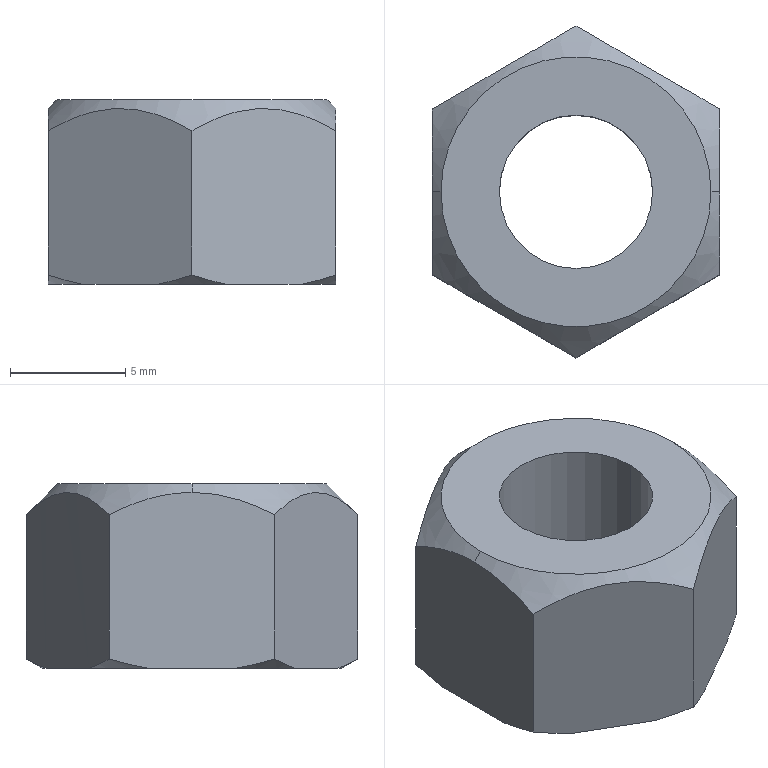Part | SolidWorks | features MBimport 1 | 1 solid | 20 faces | box 12.454 x 14.38 x 8 mm | volume 784.997 mm3 | cone 10 | plane 8 | cylinder 2 | commonest cylinder face diameters 6.647 x2
STEP:
#1=CARTESIAN_POINT('',(-5.85,0.,8.));
#2=VERTEX_POINT('',#1);
#3=CARTESIAN_POINT('',(-6.227,0.,7.623));
#4=VERTEX_POINT('',#3);
#5=CARTESIAN_POINT('',(-5.85,0.,8.));
#6=DIRECTION('',(-0.7071,0.,-0.7071));
#7=VECTOR('',#6,1000.);
#8=LINE('',#5,#7);
#9=EDGE_CURVE('',#2,#4,#8,.T.);
#10=ORIENTED_EDGE('',*,*,#9,.F.);
#11=CARTESIAN_POINT('',(5.85,0.,8.));
#12=VERTEX_POINT('',#11);
#13=CARTESIAN_POINT('',(0.,0.,8.));
#14=DIRECTION('',(0.,0.,1.));
#15=DIRECTION('',(1.,0.,0.));
#16=AXIS2_PLACEMENT_3D('',#13,#14,#15);
#17=CIRCLE('',#16,5.85);
#18=EDGE_CURVE('',#12,#2,#17,.T.);
#19=ORIENTED_EDGE('',*,*,#18,.F.);
#20=CARTESIAN_POINT('',(6.227,0.,7.623));
#21=VERTEX_POINT('',#20);
#22=CARTESIAN_POINT('',(5.85,0.,8.));
#23=DIRECTION('',(0.7071,0.,-0.7071));
#24=VECTOR('',#23,1000.);
#25=LINE('',#22,#24);
#26=EDGE_CURVE('',#12,#21,#25,.T.);
#27=ORIENTED_EDGE('',*,*,#26,.T.);
#28=CARTESIAN_POINT('',(6.227,3.595,6.66));
#29=VERTEX_POINT('',#28);
#30=CARTESIAN_POINT('',(6.227,0.,7.623));
#31=CARTESIAN_POINT('',(6.227,0.1561,7.623));
#32=CARTESIAN_POINT('',(6.227,0.3116,7.617));
#33=CARTESIAN_POINT('',(6.227,0.5452,7.6));
#34=CARTESIAN_POINT('',(6.227,0.6621,7.589));
#35=CARTESIAN_POINT('',(6.227,0.7794,7.575));
#36=CARTESIAN_POINT('',(6.227,0.8577,7.565));
#37=CARTESIAN_POINT('',(6.227,0.8982,7.559));
#38=CARTESIAN_POINT('',(6.227,1.088,7.531));
#39=CARTESIAN_POINT('',(6.227,1.24,7.503));
#40=CARTESIAN_POINT('',(6.227,1.468,7.453));
#41=CARTESIAN_POINT('',(6.227,1.582,7.426));
#42=CARTESIAN_POINT('',(6.227,1.716,7.391));
#43=CARTESIAN_POINT('',(6.227,1.774,7.376));
#44=CARTESIAN_POINT('',(6.227,1.812,7.365));
#45=CARTESIAN_POINT('',(6.227,1.833,7.359));
#46=CARTESIAN_POINT('',(6.227,2.421,7.192));
#47=CARTESIAN_POINT('',(6.227,2.994,6.96));
#48=CARTESIAN_POINT('',(6.227,3.595,6.66));
#49=B_SPLINE_CURVE_WITH_KNOTS('',3,(#30,#31,#32,#33,#34,#35,#36,#37,#38,#39,#40,#41,#42,#43,#44,#45,#46,#47,#48),.UNSPECIFIED.,.F.,.F.,(4,2,1,2,2,2,1,1,2,2,4),(0.,0.125,0.1875,0.2187,0.25,0.375,0.4375,0.4687,0.4844,0.5,1.),.UNSPECIFIED.);
#50=EDGE_CURVE('',#21,#29,#49,.T.);
#51=ORIENTED_EDGE('',*,*,#50,.T.);
#52=CARTESIAN_POINT('',(0.,7.19,6.66));
#53=VERTEX_POINT('',#52);
#54=CARTESIAN_POINT('',(6.227,3.595,6.66));
#55=CARTESIAN_POINT('',(5.969,3.744,6.809));
#56=CARTESIAN_POINT('',(5.716,3.89,6.941));
#57=CARTESIAN_POINT('',(5.343,4.105,7.114));
#58=CARTESIAN_POINT('',(5.219,4.177,7.167));
#59=CARTESIAN_POINT('',(5.034,4.283,7.24));
#60=CARTESIAN_POINT('',(4.942,4.337,7.276));
#61=CARTESIAN_POINT('',(4.835,4.399,7.314));
#62=CARTESIAN_POINT('',(4.789,4.425,7.33));
#63=CARTESIAN_POINT('',(4.758,4.443,7.34));
#64=CARTESIAN_POINT('',(4.744,4.451,7.345));
#65=CARTESIAN_POINT('',(4.595,4.537,7.394));
#66=CARTESIAN_POINT('',(4.464,4.613,7.433));
#67=CARTESIAN_POINT('',(4.267,4.726,7.483));
#68=CARTESIAN_POINT('',(4.169,4.783,7.506));
#69=CARTESIAN_POINT('',(4.071,4.84,7.526));
#70=CARTESIAN_POINT('',(4.005,4.877,7.539));
#71=CARTESIAN_POINT('',(3.974,4.896,7.545));
#72=CARTESIAN_POINT('',(3.803,4.994,7.574));
#73=CARTESIAN_POINT('',(3.668,5.072,7.592));
#74=CARTESIAN_POINT('',(3.396,5.229,7.617));
#75=CARTESIAN_POINT('',(3.26,5.308,7.623));
#76=CARTESIAN_POINT('',(2.99,5.464,7.624));
#77=CARTESIAN_POINT('',(2.856,5.541,7.618));
#78=CARTESIAN_POINT('',(2.654,5.658,7.601));
#79=CARTESIAN_POINT('',(2.587,5.697,7.594));
#80=CARTESIAN_POINT('',(2.452,5.775,7.577));
#81=CARTESIAN_POINT('',(2.382,5.815,7.567));
#82=CARTESIAN_POINT('',(2.184,5.929,7.533));
#83=CARTESIAN_POINT('',(2.052,6.006,7.505));
#84=CARTESIAN_POINT('',(1.853,6.12,7.456));
#85=CARTESIAN_POINT('',(1.753,6.178,7.429));
#86=CARTESIAN_POINT('',(1.637,6.245,7.394));
#87=CARTESIAN_POINT('',(1.587,6.274,7.379));
#88=CARTESIAN_POINT('',(1.554,6.293,7.368));
#89=CARTESIAN_POINT('',(1.536,6.303,7.362));
#90=CARTESIAN_POINT('',(1.023,6.599,7.195));
#91=CARTESIAN_POINT('',(0.5235,6.888,6.962));
#92=CARTESIAN_POINT('',(0.,7.19,6.66));
#93=B_SPLINE_CURVE_WITH_KNOTS('',3,(#54,#55,#56,#57,#58,#59,#60,#61,#62,#63,#64,#65,#66,#67,#68,#69,#70,#71,#72,#73,#74,#75,#76,#77,#78,#79,#80,#81,#82,#83,#84,#85,#86,#87,#88,#89,#90,#91,#92),.UNSPECIFIED.,.F.,.F.,(4,2,2,1,1,2,2,2,1,2,2,2,2,2,2,2,2,1,1,2,2,4),(0.,0.125,0.1875,0.2188,0.2344,0.2422,0.25,0.3125,0.3438,0.3594,0.375,0.4375,0.5,0.5625,0.5938,0.625,0.6875,0.7188,0.7344,0.7422,0.75,1.),.UNSPECIFIED.);
#94=EDGE_CURVE('',#29,#53,#93,.T.);
#95=ORIENTED_EDGE('',*,*,#94,.T.);
#96=CARTESIAN_POINT('',(-6.227,3.595,6.66));
#97=VERTEX_POINT('',#96);
#98=CARTESIAN_POINT('',(0.,7.19,6.66));
#99=CARTESIAN_POINT('',(-0.258,7.041,6.809));
#100=CARTESIAN_POINT('',(-0.5104,6.895,6.941));
#101=CARTESIAN_POINT('',(-0.884,6.679,7.114));
#102=CARTESIAN_POINT('',(-1.008,6.608,7.167));
#103=CARTESIAN_POINT('',(-1.192,6.501,7.24));
#104=CARTESIAN_POINT('',(-1.285,6.448,7.276));
#105=CARTESIAN_POINT('',(-1.392,6.386,7.314));
#106=CARTESIAN_POINT('',(-1.438,6.36,7.33));
#107=CARTESIAN_POINT('',(-1.469,6.342,7.34));
#108=CARTESIAN_POINT('',(-1.483,6.334,7.345));
#109=CARTESIAN_POINT('',(-1.632,6.248,7.394));
#110=CARTESIAN_POINT('',(-1.763,6.172,7.433));
#111=CARTESIAN_POINT('',(-1.96,6.059,7.483));
#112=CARTESIAN_POINT('',(-2.058,6.002,7.506));
#113=CARTESIAN_POINT('',(-2.156,5.945,7.526));
#114=CARTESIAN_POINT('',(-2.221,5.908,7.539));
#115=CARTESIAN_POINT('',(-2.253,5.889,7.545));
#116=CARTESIAN_POINT('',(-2.423,5.791,7.574));
#117=CARTESIAN_POINT('',(-2.559,5.712,7.592));
#118=CARTESIAN_POINT('',(-2.83,5.556,7.617));
#119=CARTESIAN_POINT('',(-2.967,5.477,7.623));
#120=CARTESIAN_POINT('',(-3.237,5.321,7.624));
#121=CARTESIAN_POINT('',(-3.371,5.244,7.618));
#122=CARTESIAN_POINT('',(-3.573,5.127,7.601));
#123=CARTESIAN_POINT('',(-3.64,5.088,7.594));
#124=CARTESIAN_POINT('',(-3.775,5.011,7.577));
#125=CARTESIAN_POINT('',(-3.844,4.971,7.567));
#126=CARTESIAN_POINT('',(-4.043,4.856,7.533));
#127=CARTESIAN_POINT('',(-4.175,4.78,7.505));
#128=CARTESIAN_POINT('',(-4.374,4.665,7.456));
#129=CARTESIAN_POINT('',(-4.473,4.607,7.429));
#130=CARTESIAN_POINT('',(-4.59,4.54,7.394));
#131=CARTESIAN_POINT('',(-4.64,4.511,7.379));
#132=CARTESIAN_POINT('',(-4.673,4.492,7.368));
#133=CARTESIAN_POINT('',(-4.691,4.482,7.362));
#134=CARTESIAN_POINT('',(-5.203,4.186,7.195));
#135=CARTESIAN_POINT('',(-5.703,3.897,6.962));
#136=CARTESIAN_POINT('',(-6.227,3.595,6.66));
#137=B_SPLINE_CURVE_WITH_KNOTS('',3,(#98,#99,#100,#101,#102,#103,#104,#105,#106,#107,#108,#109,#110,#111,#112,#113,#114,#115,#116,#117,#118,#119,#120,#121,#122,#123,#124,#125,#126,#127,#128,#129,#130,#131,#132,#133,#134,#135,#136),.UNSPECIFIED.,.F.,.F.,(4,2,2,1,1,2,2,2,1,2,2,2,2,2,2,2,2,1,1,2,2,4),(0.,0.125,0.1875,0.2187,0.2344,0.2422,0.25,0.3125,0.3437,0.3594,0.375,0.4375,0.5,0.5625,0.5937,0.625,0.6875,0.7187,0.7344,0.7422,0.75,1.),.UNSPECIFIED.);
#138=EDGE_CURVE('',#53,#97,#137,.T.);
#139=ORIENTED_EDGE('',*,*,#138,.T.);
#140=CARTESIAN_POINT('',(-6.227,3.595,6.66));
#141=CARTESIAN_POINT('',(-6.227,3.295,6.81));
#142=CARTESIAN_POINT('',(-6.227,3.001,6.943));
#143=CARTESIAN_POINT('',(-6.227,2.566,7.117));
#144=CARTESIAN_POINT('',(-6.227,2.422,7.17));
#145=CARTESIAN_POINT('',(-6.227,2.207,7.244));
#146=CARTESIAN_POINT('',(-6.227,2.1,7.279));
#147=CARTESIAN_POINT('',(-6.227,1.975,7.318));
#148=CARTESIAN_POINT('',(-6.227,1.922,7.334));
#149=CARTESIAN_POINT('',(-6.227,1.886,7.344));
#150=CARTESIAN_POINT('',(-6.227,1.87,7.349));
#151=CARTESIAN_POINT('',(-6.227,1.697,7.398));
#152=CARTESIAN_POINT('',(-6.227,1.544,7.436));
#153=CARTESIAN_POINT('',(-6.227,1.316,7.486));
#154=CARTESIAN_POINT('',(-6.227,1.202,7.509));
#155=CARTESIAN_POINT('',(-6.227,1.088,7.529));
#156=CARTESIAN_POINT('',(-6.227,1.012,7.542));
#157=CARTESIAN_POINT('',(-6.227,0.9755,7.547));
#158=CARTESIAN_POINT('',(-6.227,0.622,7.6));
#159=CARTESIAN_POINT('',(-6.227,0.3122,7.623));
#160=CARTESIAN_POINT('',(-6.227,0.,7.623));
#161=B_SPLINE_CURVE_WITH_KNOTS('',3,(#140,#141,#142,#143,#144,#145,#146,#147,#148,#149,#150,#151,#152,#153,#154,#155,#156,#157,#158,#159,#160),.UNSPECIFIED.,.F.,.F.,(4,2,2,1,1,2,2,2,1,2,2,4),(0.,0.25,0.375,0.4375,0.4688,0.4844,0.5,0.625,0.6875,0.7188,0.75,1.),.UNSPECIFIED.);
#162=EDGE_CURVE('',#97,#4,#161,.T.);
#163=ORIENTED_EDGE('',*,*,#162,.T.);
#164=EDGE_LOOP('',(#10,#19,#27,#51,#95,#139,#163));
#165=FACE_OUTER_BOUND('',#164,.T.);
#166=CARTESIAN_POINT('',(0.,0.,8.));
#167=DIRECTION('',(0.,0.,-1.));
#168=DIRECTION('',(1.,0.,0.));
#169=AXIS2_PLACEMENT_3D('',#166,#167,#168);
#170=CONICAL_SURFACE('',#169,5.85,0.7854);
#171=ADVANCED_FACE('',(#165),#170,.T.);
#172=CARTESIAN_POINT('',(3.323,0.,0.1414));
#173=VERTEX_POINT('',#172);
#174=CARTESIAN_POINT('',(3.465,0.,0.));
#175=VERTEX_POINT('',#174);
#176=CARTESIAN_POINT('',(3.465,0.,0.));
#177=DIRECTION('',(0.7071,0.,-0.7071));
#178=VECTOR('',#177,1000.);
#179=LINE('',#176,#178);
#180=EDGE_CURVE('',#173,#175,#179,.T.);
#181=ORIENTED_EDGE('',*,*,#180,.F.);
#182=CARTESIAN_POINT('',(-3.323,0.,0.1414));
#183=VERTEX_POINT('',#182);
#184=CARTESIAN_POINT('',(0.,0.,0.1414));
#185=DIRECTION('',(0.,0.,-1.));
#186=DIRECTION('',(1.,0.,0.));
#187=AXIS2_PLACEMENT_3D('',#184,#185,#186);
#188=CIRCLE('',#187,3.323);
#189=EDGE_CURVE('',#183,#173,#188,.T.);
#190=ORIENTED_EDGE('',*,*,#189,.F.);
#191=CARTESIAN_POINT('',(-3.465,0.,0.));
#192=VERTEX_POINT('',#191);
#193=CARTESIAN_POINT('',(-3.465,0.,0.));
#194=DIRECTION('',(-0.7071,0.,-0.7071));
#195=VECTOR('',#194,1000.);
#196=LINE('',#193,#195);
#197=EDGE_CURVE('',#183,#192,#196,.T.);
#198=ORIENTED_EDGE('',*,*,#197,.T.);
#199=CARTESIAN_POINT('',(0.,0.,0.));
#200=DIRECTION('',(0.,0.,1.));
#201=DIRECTION('',(1.,0.,0.));
#202=AXIS2_PLACEMENT_3D('',#199,#200,#201);
#203=CIRCLE('',#202,3.465);
#204=EDGE_CURVE('',#175,#192,#203,.T.);
#205=ORIENTED_EDGE('',*,*,#204,.F.);
#206=EDGE_LOOP('',(#181,#190,#198,#205));
#207=FACE_OUTER_BOUND('',#206,.T.);
#208=CARTESIAN_POINT('',(0.,0.,0.));
#209=DIRECTION('',(0.,0.,-1.));
#210=DIRECTION('',(-1.,0.,0.));
#211=AXIS2_PLACEMENT_3D('',#208,#209,#210);
#212=CONICAL_SURFACE('',#211,3.465,0.7854);
#213=ADVANCED_FACE('',(#207),#212,.F.);
#214=CARTESIAN_POINT('',(0.,7.19,0.3984));
#215=VERTEX_POINT('',#214);
#216=CARTESIAN_POINT('',(1.498,6.325,0.));
#217=VERTEX_POINT('',#216);
#218=CARTESIAN_POINT('',(0.,7.19,0.3984));
#219=CARTESIAN_POINT('',(0.5157,6.892,0.2265));
#220=CARTESIAN_POINT('',(1.009,6.608,0.09366));
#221=CARTESIAN_POINT('',(1.498,6.325,0.));
#222=B_SPLINE_CURVE_WITH_KNOTS('',3,(#218,#219,#220,#221),.UNSPECIFIED.,.F.,.F.,(4,4),(0.,1.),.UNSPECIFIED.);
#223=EDGE_CURVE('',#215,#217,#222,.T.);
#224=ORIENTED_EDGE('',*,*,#223,.T.);
#225=CARTESIAN_POINT('',(-1.498,6.325,0.));
#226=VERTEX_POINT('',#225);
#227=CARTESIAN_POINT('',(0.,0.,0.));
#228=DIRECTION('',(0.,0.,-1.));
#229=DIRECTION('',(-1.,0.,0.));
#230=AXIS2_PLACEMENT_3D('',#227,#228,#229);
#231=CIRCLE('',#230,6.5);
#232=EDGE_CURVE('',#226,#217,#231,.T.);
#233=ORIENTED_EDGE('',*,*,#232,.F.);
#234=CARTESIAN_POINT('',(-1.498,6.325,0.));
#235=CARTESIAN_POINT('',(-1.009,6.608,0.09366));
#236=CARTESIAN_POINT('',(-0.5157,6.892,0.2265));
#237=CARTESIAN_POINT('',(0.,7.19,0.3984));
#238=B_SPLINE_CURVE_WITH_KNOTS('',3,(#234,#235,#236,#237),.UNSPECIFIED.,.F.,.F.,(4,4),(0.,1.),.UNSPECIFIED.);
#239=EDGE_CURVE('',#226,#215,#238,.T.);
#240=ORIENTED_EDGE('',*,*,#239,.T.);
#241=EDGE_LOOP('',(#224,#233,#240));
#242=FACE_OUTER_BOUND('',#241,.T.);
#243=CARTESIAN_POINT('',(0.,0.,0.));
#244=DIRECTION('',(0.,0.,1.));
#245=DIRECTION('',(-1.,0.,0.));
#246=AXIS2_PLACEMENT_3D('',#243,#244,#245);
#247=CONICAL_SURFACE('',#246,6.5,1.047);
#248=ADVANCED_FACE('',(#242),#247,.T.);
#249=CARTESIAN_POINT('',(-6.227,3.595,0.3984));
#250=VERTEX_POINT('',#249);
#251=CARTESIAN_POINT('',(-4.728,4.46,0.));
#252=VERTEX_POINT('',#251);
#253=CARTESIAN_POINT('',(-6.227,3.595,0.3984));
#254=CARTESIAN_POINT('',(-5.711,3.893,0.2265));
#255=CARTESIAN_POINT('',(-5.218,4.177,0.09366));
#256=CARTESIAN_POINT('',(-4.728,4.46,0.));
#257=B_SPLINE_CURVE_WITH_KNOTS('',3,(#253,#254,#255,#256),.UNSPECIFIED.,.F.,.F.,(4,4),(0.,1.),.UNSPECIFIED.);
#258=EDGE_CURVE('',#250,#252,#257,.T.);
#259=ORIENTED_EDGE('',*,*,#258,.T.);
#260=CARTESIAN_POINT('',(-6.227,1.865,0.));
#261=VERTEX_POINT('',#260);
#262=CARTESIAN_POINT('',(0.,0.,0.));
#263=DIRECTION('',(0.,0.,-1.));
#264=DIRECTION('',(-1.,0.,0.));
#265=AXIS2_PLACEMENT_3D('',#262,#263,#264);
#266=CIRCLE('',#265,6.5);
#267=EDGE_CURVE('',#261,#252,#266,.T.);
#268=ORIENTED_EDGE('',*,*,#267,.F.);
#269=CARTESIAN_POINT('',(-6.227,1.865,0.));
#270=CARTESIAN_POINT('',(-6.227,2.43,0.09366));
#271=CARTESIAN_POINT('',(-6.227,2.999,0.2265));
#272=CARTESIAN_POINT('',(-6.227,3.595,0.3984));
#273=B_SPLINE_CURVE_WITH_KNOTS('',3,(#269,#270,#271,#272),.UNSPECIFIED.,.F.,.F.,(4,4),(0.,1.),.UNSPECIFIED.);
#274=EDGE_CURVE('',#261,#250,#273,.T.);
#275=ORIENTED_EDGE('',*,*,#274,.T.);
#276=EDGE_LOOP('',(#259,#268,#275));
#277=FACE_OUTER_BOUND('',#276,.T.);
#278=CARTESIAN_POINT('',(0.,0.,0.));
#279=DIRECTION('',(0.,0.,1.));
#280=DIRECTION('',(-1.,0.,0.));
#281=AXIS2_PLACEMENT_3D('',#278,#279,#280);
#282=CONICAL_SURFACE('',#281,6.5,1.047);
#283=ADVANCED_FACE('',(#277),#282,.T.);
#284=CARTESIAN_POINT('',(-6.227,-3.595,0.3984));
#285=VERTEX_POINT('',#284);
#286=CARTESIAN_POINT('',(-6.227,-1.865,0.));
#287=VERTEX_POINT('',#286);
#288=CARTESIAN_POINT('',(-6.227,-3.595,0.3984));
#289=CARTESIAN_POINT('',(-6.227,-3.022,0.2331));
#290=CARTESIAN_POINT('',(-6.227,-2.446,0.09631));
#291=CARTESIAN_POINT('',(-6.227,-1.865,0.));
#292=B_SPLINE_CURVE_WITH_KNOTS('',3,(#288,#289,#290,#291),.UNSPECIFIED.,.F.,.F.,(4,4),(0.006515,0.008293),.UNSPECIFIED.);
#293=EDGE_CURVE('',#285,#287,#292,.T.);
#294=ORIENTED_EDGE('',*,*,#293,.T.);
#295=CARTESIAN_POINT('',(-4.728,-4.46,0.));
#296=VERTEX_POINT('',#295);
#297=CARTESIAN_POINT('',(0.,0.,0.));
#298=DIRECTION('',(0.,0.,-1.));
#299=DIRECTION('',(-1.,0.,0.));
#300=AXIS2_PLACEMENT_3D('',#297,#298,#299);
#301=CIRCLE('',#300,6.5);
#302=EDGE_CURVE('',#296,#287,#301,.T.);
#303=ORIENTED_EDGE('',*,*,#302,.F.);
#304=CARTESIAN_POINT('',(-4.728,-4.46,0.));
#305=CARTESIAN_POINT('',(-5.218,-4.177,0.09366));
#306=CARTESIAN_POINT('',(-5.711,-3.893,0.2265));
#307=CARTESIAN_POINT('',(-6.227,-3.595,0.3984));
#308=B_SPLINE_CURVE_WITH_KNOTS('',3,(#304,#305,#306,#307),.UNSPECIFIED.,.F.,.F.,(4,4),(0.,1.),.UNSPECIFIED.);
#309=EDGE_CURVE('',#296,#285,#308,.T.);
#310=ORIENTED_EDGE('',*,*,#309,.T.);
#311=EDGE_LOOP('',(#294,#303,#310));
#312=FACE_OUTER_BOUND('',#311,.T.);
#313=CARTESIAN_POINT('',(0.,0.,0.));
#314=DIRECTION('',(0.,0.,1.));
#315=DIRECTION('',(-1.,0.,0.));
#316=AXIS2_PLACEMENT_3D('',#313,#314,#315);
#317=CONICAL_SURFACE('',#316,6.5,1.047);
#318=ADVANCED_FACE('',(#312),#317,.T.);
#319=CARTESIAN_POINT('',(0.,-7.19,0.3984));
#320=VERTEX_POINT('',#319);
#321=CARTESIAN_POINT('',(-1.498,-6.325,0.));
#322=VERTEX_POINT('',#321);
#323=CARTESIAN_POINT('',(0.,-7.19,0.3984));
#324=CARTESIAN_POINT('',(-0.5157,-6.892,0.2265));
#325=CARTESIAN_POINT('',(-1.009,-6.608,0.09366));
#326=CARTESIAN_POINT('',(-1.498,-6.325,0.));
#327=B_SPLINE_CURVE_WITH_KNOTS('',3,(#323,#324,#325,#326),.UNSPECIFIED.,.F.,.F.,(4,4),(0.,1.),.UNSPECIFIED.);
#328=EDGE_CURVE('',#320,#322,#327,.T.);
#329=ORIENTED_EDGE('',*,*,#328,.T.);
#330=CARTESIAN_POINT('',(1.498,-6.325,0.));
#331=VERTEX_POINT('',#330);
#332=CARTESIAN_POINT('',(0.,0.,0.));
#333=DIRECTION('',(0.,0.,-1.));
#334=DIRECTION('',(-1.,0.,0.));
#335=AXIS2_PLACEMENT_3D('',#332,#333,#334);
#336=CIRCLE('',#335,6.5);
#337=EDGE_CURVE('',#331,#322,#336,.T.);
#338=ORIENTED_EDGE('',*,*,#337,.F.);
#339=CARTESIAN_POINT('',(1.498,-6.325,0.));
#340=CARTESIAN_POINT('',(1.009,-6.608,0.09366));
#341=CARTESIAN_POINT('',(0.5157,-6.892,0.2265));
#342=CARTESIAN_POINT('',(0.,-7.19,0.3984));
#343=B_SPLINE_CURVE_WITH_KNOTS('',3,(#339,#340,#341,#342),.UNSPECIFIED.,.F.,.F.,(4,4),(0.,1.),.UNSPECIFIED.);
#344=EDGE_CURVE('',#331,#320,#343,.T.);
#345=ORIENTED_EDGE('',*,*,#344,.T.);
#346=EDGE_LOOP('',(#329,#338,#345));
#347=FACE_OUTER_BOUND('',#346,.T.);
#348=CARTESIAN_POINT('',(0.,0.,0.));
#349=DIRECTION('',(0.,0.,1.));
#350=DIRECTION('',(-1.,0.,0.));
#351=AXIS2_PLACEMENT_3D('',#348,#349,#350);
#352=CONICAL_SURFACE('',#351,6.5,1.047);
#353=ADVANCED_FACE('',(#347),#352,.T.);
#354=CARTESIAN_POINT('',(4.728,4.46,0.));
#355=VERTEX_POINT('',#354);
#356=CARTESIAN_POINT('',(6.227,3.595,0.3984));
#357=VERTEX_POINT('',#356);
#358=CARTESIAN_POINT('',(4.728,4.46,0.));
#359=CARTESIAN_POINT('',(5.218,4.177,0.09366));
#360=CARTESIAN_POINT('',(5.711,3.893,0.2265));
#361=CARTESIAN_POINT('',(6.227,3.595,0.3984));
#362=B_SPLINE_CURVE_WITH_KNOTS('',3,(#358,#359,#360,#361),.UNSPECIFIED.,.F.,.F.,(4,4),(0.,1.),.UNSPECIFIED.);
#363=EDGE_CURVE('',#355,#357,#362,.T.);
#364=ORIENTED_EDGE('',*,*,#363,.T.);
#365=CARTESIAN_POINT('',(6.227,1.865,0.));
#366=VERTEX_POINT('',#365);
#367=CARTESIAN_POINT('',(6.227,3.595,0.3984));
#368=CARTESIAN_POINT('',(6.227,3.022,0.2331));
#369=CARTESIAN_POINT('',(6.227,2.446,0.09631));
#370=CARTESIAN_POINT('',(6.227,1.865,0.));
#371=B_SPLINE_CURVE_WITH_KNOTS('',3,(#367,#368,#369,#370),.UNSPECIFIED.,.F.,.F.,(4,4),(0.006515,0.008293),.UNSPECIFIED.);
#372=EDGE_CURVE('',#357,#366,#371,.T.);
#373=ORIENTED_EDGE('',*,*,#372,.T.);
#374=CARTESIAN_POINT('',(0.,0.,0.));
#375=DIRECTION('',(0.,0.,-1.));
#376=DIRECTION('',(-1.,0.,0.));
#377=AXIS2_PLACEMENT_3D('',#374,#375,#376);
#378=CIRCLE('',#377,6.5);
#379=EDGE_CURVE('',#355,#366,#378,.T.);
#380=ORIENTED_EDGE('',*,*,#379,.F.);
#381=EDGE_LOOP('',(#364,#373,#380));
#382=FACE_OUTER_BOUND('',#381,.T.);
#383=CARTESIAN_POINT('',(0.,0.,0.));
#384=DIRECTION('',(0.,0.,1.));
#385=DIRECTION('',(-1.,0.,0.));
#386=AXIS2_PLACEMENT_3D('',#383,#384,#385);
#387=CONICAL_SURFACE('',#386,6.5,1.047);
#388=ADVANCED_FACE('',(#382),#387,.T.);
#389=CARTESIAN_POINT('',(6.227,-3.595,0.3984));
#390=VERTEX_POINT('',#389);
#391=CARTESIAN_POINT('',(4.728,-4.46,0.));
#392=VERTEX_POINT('',#391);
#393=CARTESIAN_POINT('',(6.227,-3.595,0.3984));
#394=CARTESIAN_POINT('',(5.711,-3.893,0.2265));
#395=CARTESIAN_POINT('',(5.218,-4.177,0.09366));
#396=CARTESIAN_POINT('',(4.728,-4.46,0.));
#397=B_SPLINE_CURVE_WITH_KNOTS('',3,(#393,#394,#395,#396),.UNSPECIFIED.,.F.,.F.,(4,4),(0.,1.),.UNSPECIFIED.);
#398=EDGE_CURVE('',#390,#392,#397,.T.);
#399=ORIENTED_EDGE('',*,*,#398,.T.);
#400=CARTESIAN_POINT('',(6.227,-1.865,0.));
#401=VERTEX_POINT('',#400);
#402=CARTESIAN_POINT('',(0.,0.,0.));
#403=DIRECTION('',(0.,0.,-1.));
#404=DIRECTION('',(-1.,0.,0.));
#405=AXIS2_PLACEMENT_3D('',#402,#403,#404);
#406=CIRCLE('',#405,6.5);
#407=EDGE_CURVE('',#401,#392,#406,.T.);
#408=ORIENTED_EDGE('',*,*,#407,.F.);
#409=CARTESIAN_POINT('',(6.227,-1.865,0.));
#410=CARTESIAN_POINT('',(6.227,-2.43,0.09366));
#411=CARTESIAN_POINT('',(6.227,-2.999,0.2265));
#412=CARTESIAN_POINT('',(6.227,-3.595,0.3984));
#413=B_SPLINE_CURVE_WITH_KNOTS('',3,(#409,#410,#411,#412),.UNSPECIFIED.,.F.,.F.,(4,4),(0.,1.),.UNSPECIFIED.);
#414=EDGE_CURVE('',#401,#390,#413,.T.);
#415=ORIENTED_EDGE('',*,*,#414,.T.);
#416=EDGE_LOOP('',(#399,#408,#415));
#417=FACE_OUTER_BOUND('',#416,.T.);
#418=CARTESIAN_POINT('',(0.,0.,0.));
#419=DIRECTION('',(0.,0.,1.));
#420=DIRECTION('',(-1.,0.,0.));
#421=AXIS2_PLACEMENT_3D('',#418,#419,#420);
#422=CONICAL_SURFACE('',#421,6.5,1.047);
#423=ADVANCED_FACE('',(#417),#422,.T.);
#424=CARTESIAN_POINT('',(3.323,0.,8.));
#425=VERTEX_POINT('',#424);
#426=CARTESIAN_POINT('',(3.323,0.,8.));
#427=DIRECTION('',(0.,0.,-1.));
#428=VECTOR('',#427,1000.);
#429=LINE('',#426,#428);
#430=EDGE_CURVE('',#425,#173,#429,.T.);
#431=ORIENTED_EDGE('',*,*,#430,.F.);
#432=CARTESIAN_POINT('',(-3.323,0.,8.));
#433=VERTEX_POINT('',#432);
#434=CARTESIAN_POINT('',(0.,0.,8.));
#435=DIRECTION('',(0.,0.,1.));
#436=DIRECTION('',(1.,0.,0.));
#437=AXIS2_PLACEMENT_3D('',#434,#435,#436);
#438=CIRCLE('',#437,3.323);
#439=EDGE_CURVE('',#425,#433,#438,.T.);
#440=ORIENTED_EDGE('',*,*,#439,.T.);
#441=CARTESIAN_POINT('',(-3.323,0.,8.));
#442=DIRECTION('',(0.,0.,-1.));
#443=VECTOR('',#442,1000.);
#444=LINE('',#441,#443);
#445=EDGE_CURVE('',#433,#183,#444,.T.);
#446=ORIENTED_EDGE('',*,*,#445,.T.);
#447=ORIENTED_EDGE('',*,*,#189,.T.);
#448=EDGE_LOOP('',(#431,#440,#446,#447));
#449=FACE_OUTER_BOUND('',#448,.T.);
#450=CARTESIAN_POINT('',(0.,0.,8.));
#451=DIRECTION('',(0.,0.,-1.));
#452=DIRECTION('',(-1.,0.,0.));
#453=AXIS2_PLACEMENT_3D('',#450,#451,#452);
#454=CYLINDRICAL_SURFACE('',#453,3.323);
#455=ADVANCED_FACE('',(#449),#454,.F.);
#456=CARTESIAN_POINT('',(0.,0.,0.));
#457=DIRECTION('',(0.,0.,1.));
#458=DIRECTION('',(1.,0.,0.));
#459=AXIS2_PLACEMENT_3D('',#456,#457,#458);
#460=CIRCLE('',#459,3.465);
#461=EDGE_CURVE('',#192,#175,#460,.T.);
#462=ORIENTED_EDGE('',*,*,#461,.T.);
#463=ORIENTED_EDGE('',*,*,#204,.T.);
#464=EDGE_LOOP('',(#462,#463));
#465=FACE_BOUND('',#464,.T.);
#466=ORIENTED_EDGE('',*,*,#379,.T.);
#467=CARTESIAN_POINT('',(6.227,-3.595,0.));
#468=DIRECTION('',(0.,1.,0.));
#469=VECTOR('',#468,1000.);
#470=LINE('',#467,#469);
#471=EDGE_CURVE('',#401,#366,#470,.T.);
#472=ORIENTED_EDGE('',*,*,#471,.F.);
#473=ORIENTED_EDGE('',*,*,#407,.T.);
#474=CARTESIAN_POINT('',(0.,-7.19,0.));
#475=DIRECTION('',(0.866,0.5,0.));
#476=VECTOR('',#475,1000.);
#477=LINE('',#474,#476);
#478=EDGE_CURVE('',#331,#392,#477,.T.);
#479=ORIENTED_EDGE('',*,*,#478,.F.);
#480=ORIENTED_EDGE('',*,*,#337,.T.);
#481=CARTESIAN_POINT('',(-6.227,-3.595,0.));
#482=DIRECTION('',(0.866,-0.5,0.));
#483=VECTOR('',#482,1000.);
#484=LINE('',#481,#483);
#485=EDGE_CURVE('',#296,#322,#484,.T.);
#486=ORIENTED_EDGE('',*,*,#485,.F.);
#487=ORIENTED_EDGE('',*,*,#302,.T.);
#488=CARTESIAN_POINT('',(-6.227,3.595,0.));
#489=DIRECTION('',(0.,-1.,0.));
#490=VECTOR('',#489,1000.);
#491=LINE('',#488,#490);
#492=EDGE_CURVE('',#261,#287,#491,.T.);
#493=ORIENTED_EDGE('',*,*,#492,.F.);
#494=ORIENTED_EDGE('',*,*,#267,.T.);
#495=CARTESIAN_POINT('',(0.,7.19,0.));
#496=DIRECTION('',(-0.866,-0.5,0.));
#497=VECTOR('',#496,1000.);
#498=LINE('',#495,#497);
#499=EDGE_CURVE('',#226,#252,#498,.T.);
#500=ORIENTED_EDGE('',*,*,#499,.F.);
#501=ORIENTED_EDGE('',*,*,#232,.T.);
#502=CARTESIAN_POINT('',(6.227,3.595,0.));
#503=DIRECTION('',(-0.866,0.5,0.));
#504=VECTOR('',#503,1000.);
#505=LINE('',#502,#504);
#506=EDGE_CURVE('',#355,#217,#505,.T.);
#507=ORIENTED_EDGE('',*,*,#506,.F.);
#508=EDGE_LOOP('',(#466,#472,#473,#479,#480,#486,#487,#493,#494,#500,#501,#507));
#509=FACE_OUTER_BOUND('',#508,.T.);
#510=CARTESIAN_POINT('',(-6.227,10.785,0.));
#511=DIRECTION('',(0.,0.,1.));
#512=DIRECTION('',(1.,0.,0.));
#513=AXIS2_PLACEMENT_3D('',#510,#511,#512);
#514=PLANE('',#513);
#515=ADVANCED_FACE('',(#465,#509),#514,.F.);
#516=CARTESIAN_POINT('',(0.,0.,8.));
#517=DIRECTION('',(0.,0.,1.));
#518=DIRECTION('',(1.,0.,0.));
#519=AXIS2_PLACEMENT_3D('',#516,#517,#518);
#520=CIRCLE('',#519,3.323);
#521=EDGE_CURVE('',#433,#425,#520,.T.);
#522=ORIENTED_EDGE('',*,*,#521,.F.);
#523=ORIENTED_EDGE('',*,*,#439,.F.);
#524=EDGE_LOOP('',(#522,#523));
#525=FACE_BOUND('',#524,.T.);
#526=ORIENTED_EDGE('',*,*,#18,.T.);
#527=CARTESIAN_POINT('',(0.,0.,8.));
#528=DIRECTION('',(0.,0.,1.));
#529=DIRECTION('',(1.,0.,0.));
#530=AXIS2_PLACEMENT_3D('',#527,#528,#529);
#531=CIRCLE('',#530,5.85);
#532=EDGE_CURVE('',#2,#12,#531,.T.);
#533=ORIENTED_EDGE('',*,*,#532,.T.);
#534=EDGE_LOOP('',(#526,#533));
#535=FACE_OUTER_BOUND('',#534,.T.);
#536=CARTESIAN_POINT('',(-6.227,10.785,8.));
#537=DIRECTION('',(0.,0.,1.));
#538=DIRECTION('',(1.,0.,0.));
#539=AXIS2_PLACEMENT_3D('',#536,#537,#538);
#540=PLANE('',#539);
#541=ADVANCED_FACE('',(#525,#535),#540,.T.);
#542=CARTESIAN_POINT('',(6.227,-3.595,6.66));
#543=VERTEX_POINT('',#542);
#544=CARTESIAN_POINT('',(6.227,-3.595,6.66));
#545=CARTESIAN_POINT('',(6.227,-3.295,6.81));
#546=CARTESIAN_POINT('',(6.227,-3.001,6.943));
#547=CARTESIAN_POINT('',(6.227,-2.567,7.116));
#548=CARTESIAN_POINT('',(6.227,-2.423,7.17));
#549=CARTESIAN_POINT('',(6.227,-2.208,7.244));
#550=CARTESIAN_POINT('',(6.227,-2.101,7.279));
#551=CARTESIAN_POINT('',(6.227,-1.976,7.317));
#552=CARTESIAN_POINT('',(6.227,-1.922,7.333));
#553=CARTESIAN_POINT('',(6.227,-1.887,7.344));
#554=CARTESIAN_POINT('',(6.227,-1.87,7.349));
#555=CARTESIAN_POINT('',(6.227,-1.698,7.398));
#556=CARTESIAN_POINT('',(6.227,-1.545,7.436));
#557=CARTESIAN_POINT('',(6.227,-1.318,7.486));
#558=CARTESIAN_POINT('',(6.227,-1.204,7.509));
#559=CARTESIAN_POINT('',(6.227,-1.091,7.529));
#560=CARTESIAN_POINT('',(6.227,-1.015,7.541));
#561=CARTESIAN_POINT('',(6.227,-0.9785,7.547));
#562=CARTESIAN_POINT('',(6.227,-0.6244,7.6));
#563=CARTESIAN_POINT('',(6.227,-0.3136,7.623));
#564=CARTESIAN_POINT('',(6.227,0.,7.623));
#565=B_SPLINE_CURVE_WITH_KNOTS('',3,(#544,#545,#546,#547,#548,#549,#550,#551,#552,#553,#554,#555,#556,#557,#558,#559,#560,#561,#562,#563,#564),.UNSPECIFIED.,.F.,.F.,(4,2,2,1,1,2,2,2,1,2,2,4),(0.,0.25,0.375,0.4375,0.4688,0.4844,0.5,0.625,0.6875,0.7188,0.75,1.),.UNSPECIFIED.);
#566=EDGE_CURVE('',#543,#21,#565,.T.);
#567=ORIENTED_EDGE('',*,*,#566,.F.);
#568=CARTESIAN_POINT('',(6.227,-3.595,8.));
#569=DIRECTION('',(0.,0.,-1.));
#570=VECTOR('',#569,1000.);
#571=LINE('',#568,#570);
#572=EDGE_CURVE('',#543,#390,#571,.T.);
#573=ORIENTED_EDGE('',*,*,#572,.T.);
#574=ORIENTED_EDGE('',*,*,#414,.F.);
#575=ORIENTED_EDGE('',*,*,#471,.T.);
#576=ORIENTED_EDGE('',*,*,#372,.F.);
#577=CARTESIAN_POINT('',(6.227,3.595,8.));
#578=DIRECTION('',(0.,0.,-1.));
#579=VECTOR('',#578,1000.);
#580=LINE('',#577,#579);
#581=EDGE_CURVE('',#29,#357,#580,.T.);
#582=ORIENTED_EDGE('',*,*,#581,.F.);
#583=ORIENTED_EDGE('',*,*,#50,.F.);
#584=EDGE_LOOP('',(#567,#573,#574,#575,#576,#582,#583));
#585=FACE_OUTER_BOUND('',#584,.T.);
#586=CARTESIAN_POINT('',(6.227,-3.595,8.));
#587=DIRECTION('',(-1.,0.,0.));
#588=DIRECTION('',(0.,1.,0.));
#589=AXIS2_PLACEMENT_3D('',#586,#587,#588);
#590=PLANE('',#589);
#591=ADVANCED_FACE('',(#585),#590,.F.);
#592=CARTESIAN_POINT('',(0.,-7.19,6.66));
#593=VERTEX_POINT('',#592);
#594=CARTESIAN_POINT('',(0.,-7.19,6.66));
#595=CARTESIAN_POINT('',(0.258,-7.041,6.809));
#596=CARTESIAN_POINT('',(0.5104,-6.895,6.941));
#597=CARTESIAN_POINT('',(0.884,-6.679,7.114));
#598=CARTESIAN_POINT('',(1.008,-6.608,7.167));
#599=CARTESIAN_POINT('',(1.192,-6.501,7.24));
#600=CARTESIAN_POINT('',(1.285,-6.448,7.276));
#601=CARTESIAN_POINT('',(1.392,-6.386,7.314));
#602=CARTESIAN_POINT('',(1.438,-6.36,7.33));
#603=CARTESIAN_POINT('',(1.469,-6.342,7.34));
#604=CARTESIAN_POINT('',(1.483,-6.334,7.345));
#605=CARTESIAN_POINT('',(1.632,-6.248,7.394));
#606=CARTESIAN_POINT('',(1.763,-6.172,7.433));
#607=CARTESIAN_POINT('',(1.96,-6.059,7.483));
#608=CARTESIAN_POINT('',(2.058,-6.002,7.506));
#609=CARTESIAN_POINT('',(2.156,-5.945,7.526));
#610=CARTESIAN_POINT('',(2.221,-5.908,7.539));
#611=CARTESIAN_POINT('',(2.253,-5.889,7.545));
#612=CARTESIAN_POINT('',(2.423,-5.791,7.574));
#613=CARTESIAN_POINT('',(2.559,-5.712,7.592));
#614=CARTESIAN_POINT('',(2.83,-5.556,7.617));
#615=CARTESIAN_POINT('',(2.967,-5.477,7.623));
#616=CARTESIAN_POINT('',(3.237,-5.321,7.624));
#617=CARTESIAN_POINT('',(3.371,-5.244,7.618));
#618=CARTESIAN_POINT('',(3.573,-5.127,7.601));
#619=CARTESIAN_POINT('',(3.64,-5.088,7.594));
#620=CARTESIAN_POINT('',(3.775,-5.011,7.577));
#621=CARTESIAN_POINT('',(3.844,-4.971,7.567));
#622=CARTESIAN_POINT('',(4.043,-4.856,7.533));
#623=CARTESIAN_POINT('',(4.175,-4.78,7.505));
#624=CARTESIAN_POINT('',(4.374,-4.665,7.456));
#625=CARTESIAN_POINT('',(4.473,-4.607,7.429));
#626=CARTESIAN_POINT('',(4.59,-4.54,7.394));
#627=CARTESIAN_POINT('',(4.64,-4.511,7.379));
#628=CARTESIAN_POINT('',(4.673,-4.492,7.368));
#629=CARTESIAN_POINT('',(4.691,-4.482,7.362));
#630=CARTESIAN_POINT('',(5.203,-4.186,7.195));
#631=CARTESIAN_POINT('',(5.703,-3.897,6.962));
#632=CARTESIAN_POINT('',(6.227,-3.595,6.66));
#633=B_SPLINE_CURVE_WITH_KNOTS('',3,(#594,#595,#596,#597,#598,#599,#600,#601,#602,#603,#604,#605,#606,#607,#608,#609,#610,#611,#612,#613,#614,#615,#616,#617,#618,#619,#620,#621,#622,#623,#624,#625,#626,#627,#628,#629,#630,#631,#632),.UNSPECIFIED.,.F.,.F.,(4,2,2,1,1,2,2,2,1,2,2,2,2,2,2,2,2,1,1,2,2,4),(0.,0.125,0.1875,0.2187,0.2344,0.2422,0.25,0.3125,0.3437,0.3594,0.375,0.4375,0.5,0.5625,0.5937,0.625,0.6875,0.7188,0.7344,0.7422,0.75,1.),.UNSPECIFIED.);
#634=EDGE_CURVE('',#593,#543,#633,.T.);
#635=ORIENTED_EDGE('',*,*,#634,.F.);
#636=CARTESIAN_POINT('',(0.,-7.19,8.));
#637=DIRECTION('',(0.,0.,-1.));
#638=VECTOR('',#637,1000.);
#639=LINE('',#636,#638);
#640=EDGE_CURVE('',#593,#320,#639,.T.);
#641=ORIENTED_EDGE('',*,*,#640,.T.);
#642=ORIENTED_EDGE('',*,*,#344,.F.);
#643=ORIENTED_EDGE('',*,*,#478,.T.);
#644=ORIENTED_EDGE('',*,*,#398,.F.);
#645=ORIENTED_EDGE('',*,*,#572,.F.);
#646=EDGE_LOOP('',(#635,#641,#642,#643,#644,#645));
#647=FACE_OUTER_BOUND('',#646,.T.);
#648=CARTESIAN_POINT('',(0.,-7.19,8.));
#649=DIRECTION('',(-0.5,0.866,0.));
#650=DIRECTION('',(0.,0.,1.));
#651=AXIS2_PLACEMENT_3D('',#648,#649,#650);
#652=PLANE('',#651);
#653=ADVANCED_FACE('',(#647),#652,.F.);
#654=CARTESIAN_POINT('',(-6.227,-3.595,6.66));
#655=VERTEX_POINT('',#654);
#656=CARTESIAN_POINT('',(-6.227,-3.595,6.66));
#657=CARTESIAN_POINT('',(-5.969,-3.744,6.809));
#658=CARTESIAN_POINT('',(-5.716,-3.89,6.941));
#659=CARTESIAN_POINT('',(-5.343,-4.105,7.114));
#660=CARTESIAN_POINT('',(-5.219,-4.177,7.167));
#661=CARTESIAN_POINT('',(-5.034,-4.283,7.24));
#662=CARTESIAN_POINT('',(-4.942,-4.337,7.276));
#663=CARTESIAN_POINT('',(-4.835,-4.399,7.314));
#664=CARTESIAN_POINT('',(-4.789,-4.425,7.33));
#665=CARTESIAN_POINT('',(-4.758,-4.443,7.34));
#666=CARTESIAN_POINT('',(-4.744,-4.451,7.345));
#667=CARTESIAN_POINT('',(-4.595,-4.537,7.394));
#668=CARTESIAN_POINT('',(-4.464,-4.613,7.433));
#669=CARTESIAN_POINT('',(-4.267,-4.726,7.483));
#670=CARTESIAN_POINT('',(-4.169,-4.783,7.506));
#671=CARTESIAN_POINT('',(-4.071,-4.84,7.526));
#672=CARTESIAN_POINT('',(-4.005,-4.877,7.539));
#673=CARTESIAN_POINT('',(-3.974,-4.896,7.545));
#674=CARTESIAN_POINT('',(-3.803,-4.994,7.574));
#675=CARTESIAN_POINT('',(-3.668,-5.072,7.592));
#676=CARTESIAN_POINT('',(-3.396,-5.229,7.617));
#677=CARTESIAN_POINT('',(-3.26,-5.308,7.623));
#678=CARTESIAN_POINT('',(-2.99,-5.464,7.624));
#679=CARTESIAN_POINT('',(-2.856,-5.541,7.618));
#680=CARTESIAN_POINT('',(-2.654,-5.658,7.601));
#681=CARTESIAN_POINT('',(-2.587,-5.697,7.594));
#682=CARTESIAN_POINT('',(-2.452,-5.775,7.577));
#683=CARTESIAN_POINT('',(-2.382,-5.815,7.567));
#684=CARTESIAN_POINT('',(-2.184,-5.929,7.533));
#685=CARTESIAN_POINT('',(-2.052,-6.006,7.505));
#686=CARTESIAN_POINT('',(-1.853,-6.12,7.456));
#687=CARTESIAN_POINT('',(-1.753,-6.178,7.429));
#688=CARTESIAN_POINT('',(-1.637,-6.245,7.394));
#689=CARTESIAN_POINT('',(-1.587,-6.274,7.379));
#690=CARTESIAN_POINT('',(-1.554,-6.293,7.368));
#691=CARTESIAN_POINT('',(-1.536,-6.303,7.362));
#692=CARTESIAN_POINT('',(-1.023,-6.599,7.195));
#693=CARTESIAN_POINT('',(-0.5235,-6.888,6.962));
#694=CARTESIAN_POINT('',(0.,-7.19,6.66));
#695=B_SPLINE_CURVE_WITH_KNOTS('',3,(#656,#657,#658,#659,#660,#661,#662,#663,#664,#665,#666,#667,#668,#669,#670,#671,#672,#673,#674,#675,#676,#677,#678,#679,#680,#681,#682,#683,#684,#685,#686,#687,#688,#689,#690,#691,#692,#693,#694),.UNSPECIFIED.,.F.,.F.,(4,2,2,1,1,2,2,2,1,2,2,2,2,2,2,2,2,1,1,2,2,4),(0.,0.125,0.1875,0.2188,0.2344,0.2422,0.25,0.3125,0.3437,0.3594,0.375,0.4375,0.5,0.5625,0.5937,0.625,0.6875,0.7187,0.7344,0.7422,0.75,1.),.UNSPECIFIED.);
#696=EDGE_CURVE('',#655,#593,#695,.T.);
#697=ORIENTED_EDGE('',*,*,#696,.F.);
#698=CARTESIAN_POINT('',(-6.227,-3.595,8.));
#699=DIRECTION('',(0.,0.,-1.));
#700=VECTOR('',#699,1000.);
#701=LINE('',#698,#700);
#702=EDGE_CURVE('',#655,#285,#701,.T.);
#703=ORIENTED_EDGE('',*,*,#702,.T.);
#704=ORIENTED_EDGE('',*,*,#309,.F.);
#705=ORIENTED_EDGE('',*,*,#485,.T.);
#706=ORIENTED_EDGE('',*,*,#328,.F.);
#707=ORIENTED_EDGE('',*,*,#640,.F.);
#708=EDGE_LOOP('',(#697,#703,#704,#705,#706,#707));
#709=FACE_OUTER_BOUND('',#708,.T.);
#710=CARTESIAN_POINT('',(-6.227,-3.595,8.));
#711=DIRECTION('',(0.5,0.866,0.));
#712=DIRECTION('',(0.,0.,-1.));
#713=AXIS2_PLACEMENT_3D('',#710,#711,#712);
#714=PLANE('',#713);
#715=ADVANCED_FACE('',(#709),#714,.F.);
#716=ORIENTED_EDGE('',*,*,#162,.F.);
#717=CARTESIAN_POINT('',(-6.227,3.595,8.));
#718=DIRECTION('',(0.,0.,-1.));
#719=VECTOR('',#718,1000.);
#720=LINE('',#717,#719);
#721=EDGE_CURVE('',#97,#250,#720,.T.);
#722=ORIENTED_EDGE('',*,*,#721,.T.);
#723=ORIENTED_EDGE('',*,*,#274,.F.);
#724=ORIENTED_EDGE('',*,*,#492,.T.);
#725=ORIENTED_EDGE('',*,*,#293,.F.);
#726=ORIENTED_EDGE('',*,*,#702,.F.);
#727=CARTESIAN_POINT('',(-6.227,0.,7.623));
#728=CARTESIAN_POINT('',(-6.227,-0.1568,7.623));
#729=CARTESIAN_POINT('',(-6.227,-0.3129,7.617));
#730=CARTESIAN_POINT('',(-6.227,-0.5472,7.6));
#731=CARTESIAN_POINT('',(-6.227,-0.6645,7.589));
#732=CARTESIAN_POINT('',(-6.227,-0.782,7.574));
#733=CARTESIAN_POINT('',(-6.227,-0.8605,7.564));
#734=CARTESIAN_POINT('',(-6.227,-0.9013,7.558));
#735=CARTESIAN_POINT('',(-6.227,-1.091,7.53));
#736=CARTESIAN_POINT('',(-6.227,-1.242,7.502));
#737=CARTESIAN_POINT('',(-6.227,-1.47,7.453));
#738=CARTESIAN_POINT('',(-6.227,-1.584,7.426));
#739=CARTESIAN_POINT('',(-6.227,-1.717,7.391));
#740=CARTESIAN_POINT('',(-6.227,-1.774,7.375));
#741=CARTESIAN_POINT('',(-6.227,-1.813,7.365));
#742=CARTESIAN_POINT('',(-6.227,-1.833,7.359));
#743=CARTESIAN_POINT('',(-6.227,-2.421,7.192));
#744=CARTESIAN_POINT('',(-6.227,-2.995,6.96));
#745=CARTESIAN_POINT('',(-6.227,-3.595,6.66));
#746=B_SPLINE_CURVE_WITH_KNOTS('',3,(#727,#728,#729,#730,#731,#732,#733,#734,#735,#736,#737,#738,#739,#740,#741,#742,#743,#744,#745),.UNSPECIFIED.,.F.,.F.,(4,2,1,2,2,2,1,1,2,2,4),(0.,0.125,0.1875,0.2188,0.25,0.375,0.4375,0.4688,0.4844,0.5,1.),.UNSPECIFIED.);
#747=EDGE_CURVE('',#4,#655,#746,.T.);
#748=ORIENTED_EDGE('',*,*,#747,.F.);
#749=EDGE_LOOP('',(#716,#722,#723,#724,#725,#726,#748));
#750=FACE_OUTER_BOUND('',#749,.T.);
#751=CARTESIAN_POINT('',(-6.227,3.595,8.));
#752=DIRECTION('',(1.,0.,0.));
#753=DIRECTION('',(0.,1.,0.));
#754=AXIS2_PLACEMENT_3D('',#751,#752,#753);
#755=PLANE('',#754);
#756=ADVANCED_FACE('',(#750),#755,.F.);
#757=ORIENTED_EDGE('',*,*,#138,.F.);
#758=CARTESIAN_POINT('',(0.,7.19,8.));
#759=DIRECTION('',(0.,0.,-1.));
#760=VECTOR('',#759,1000.);
#761=LINE('',#758,#760);
#762=EDGE_CURVE('',#53,#215,#761,.T.);
#763=ORIENTED_EDGE('',*,*,#762,.T.);
#764=ORIENTED_EDGE('',*,*,#239,.F.);
#765=ORIENTED_EDGE('',*,*,#499,.T.);
#766=ORIENTED_EDGE('',*,*,#258,.F.);
#767=ORIENTED_EDGE('',*,*,#721,.F.);
#768=EDGE_LOOP('',(#757,#763,#764,#765,#766,#767));
#769=FACE_OUTER_BOUND('',#768,.T.);
#770=CARTESIAN_POINT('',(0.,7.19,8.));
#771=DIRECTION('',(0.5,-0.866,0.));
#772=DIRECTION('',(0.,0.,-1.));
#773=AXIS2_PLACEMENT_3D('',#770,#771,#772);
#774=PLANE('',#773);
#775=ADVANCED_FACE('',(#769),#774,.F.);
#776=ORIENTED_EDGE('',*,*,#94,.F.);
#777=ORIENTED_EDGE('',*,*,#581,.T.);
#778=ORIENTED_EDGE('',*,*,#363,.F.);
#779=ORIENTED_EDGE('',*,*,#506,.T.);
#780=ORIENTED_EDGE('',*,*,#223,.F.);
#781=ORIENTED_EDGE('',*,*,#762,.F.);
#782=EDGE_LOOP('',(#776,#777,#778,#779,#780,#781));
#783=FACE_OUTER_BOUND('',#782,.T.);
#784=CARTESIAN_POINT('',(6.227,3.595,8.));
#785=DIRECTION('',(-0.5,-0.866,0.));
#786=DIRECTION('',(-0.866,0.5,0.));
#787=AXIS2_PLACEMENT_3D('',#784,#785,#786);
#788=PLANE('',#787);
#789=ADVANCED_FACE('',(#783),#788,.F.);
#790=ORIENTED_EDGE('',*,*,#521,.T.);
#791=ORIENTED_EDGE('',*,*,#430,.T.);
#792=CARTESIAN_POINT('',(0.,0.,0.1414));
#793=DIRECTION('',(0.,0.,-1.));
#794=DIRECTION('',(1.,0.,0.));
#795=AXIS2_PLACEMENT_3D('',#792,#793,#794);
#796=CIRCLE('',#795,3.323);
#797=EDGE_CURVE('',#173,#183,#796,.T.);
#798=ORIENTED_EDGE('',*,*,#797,.T.);
#799=ORIENTED_EDGE('',*,*,#445,.F.);
#800=EDGE_LOOP('',(#790,#791,#798,#799));
#801=FACE_OUTER_BOUND('',#800,.T.);
#802=CARTESIAN_POINT('',(0.,0.,8.));
#803=DIRECTION('',(0.,0.,-1.));
#804=DIRECTION('',(-1.,0.,0.));
#805=AXIS2_PLACEMENT_3D('',#802,#803,#804);
#806=CYLINDRICAL_SURFACE('',#805,3.323);
#807=ADVANCED_FACE('',(#801),#806,.F.);
#808=ORIENTED_EDGE('',*,*,#797,.F.);
#809=ORIENTED_EDGE('',*,*,#180,.T.);
#810=ORIENTED_EDGE('',*,*,#461,.F.);
#811=ORIENTED_EDGE('',*,*,#197,.F.);
#812=EDGE_LOOP('',(#808,#809,#810,#811));
#813=FACE_OUTER_BOUND('',#812,.T.);
#814=CARTESIAN_POINT('',(0.,0.,0.));
#815=DIRECTION('',(0.,0.,-1.));
#816=DIRECTION('',(-1.,0.,0.));
#817=AXIS2_PLACEMENT_3D('',#814,#815,#816);
#818=CONICAL_SURFACE('',#817,3.465,0.7854);
#819=ADVANCED_FACE('',(#813),#818,.F.);
#820=ORIENTED_EDGE('',*,*,#532,.F.);
#821=ORIENTED_EDGE('',*,*,#9,.T.);
#822=ORIENTED_EDGE('',*,*,#747,.T.);
#823=ORIENTED_EDGE('',*,*,#696,.T.);
#824=ORIENTED_EDGE('',*,*,#634,.T.);
#825=ORIENTED_EDGE('',*,*,#566,.T.);
#826=ORIENTED_EDGE('',*,*,#26,.F.);
#827=EDGE_LOOP('',(#820,#821,#822,#823,#824,#825,#826));
#828=FACE_OUTER_BOUND('',#827,.T.);
#829=CARTESIAN_POINT('',(0.,0.,8.));
#830=DIRECTION('',(0.,0.,-1.));
#831=DIRECTION('',(1.,0.,0.));
#832=AXIS2_PLACEMENT_3D('',#829,#830,#831);
#833=CONICAL_SURFACE('',#832,5.85,0.7854);
#834=ADVANCED_FACE('',(#828),#833,.T.);
#835=CLOSED_SHELL('',(#171,#213,#248,#283,#318,#353,#388,#423,#455,#515,#541,#591,#653,#715,#756,#775,#789,#807,#819,#834));
#836=MANIFOLD_SOLID_BREP('',#835);
#837=CARTESIAN_POINT('',(0.,0.,0.));
#838=DIRECTION('',(0.,0.,1.));
#839=DIRECTION('',(1.,0.,0.));
#840=AXIS2_PLACEMENT_3D('',#837,#838,#839);
#841=(LENGTH_UNIT()NAMED_UNIT(*)SI_UNIT(.MILLI.,.METRE.));
#842=UNCERTAINTY_MEASURE_WITH_UNIT(LENGTH_MEASURE(0.00001),#841,'','');
#843=(NAMED_UNIT(*)PLANE_ANGLE_UNIT()SI_UNIT($,.RADIAN.));
#844=(NAMED_UNIT(*)SI_UNIT($,.STERADIAN.)SOLID_ANGLE_UNIT());
#845=(GEOMETRIC_REPRESENTATION_CONTEXT(3)GLOBAL_UNCERTAINTY_ASSIGNED_CONTEXT((#842))GLOBAL_UNIT_ASSIGNED_CONTEXT((#841,#843,#844))REPRESENTATION_CONTEXT('',''));
#846=ADVANCED_BREP_SHAPE_REPRESENTATION('',(#836,#840),#845);